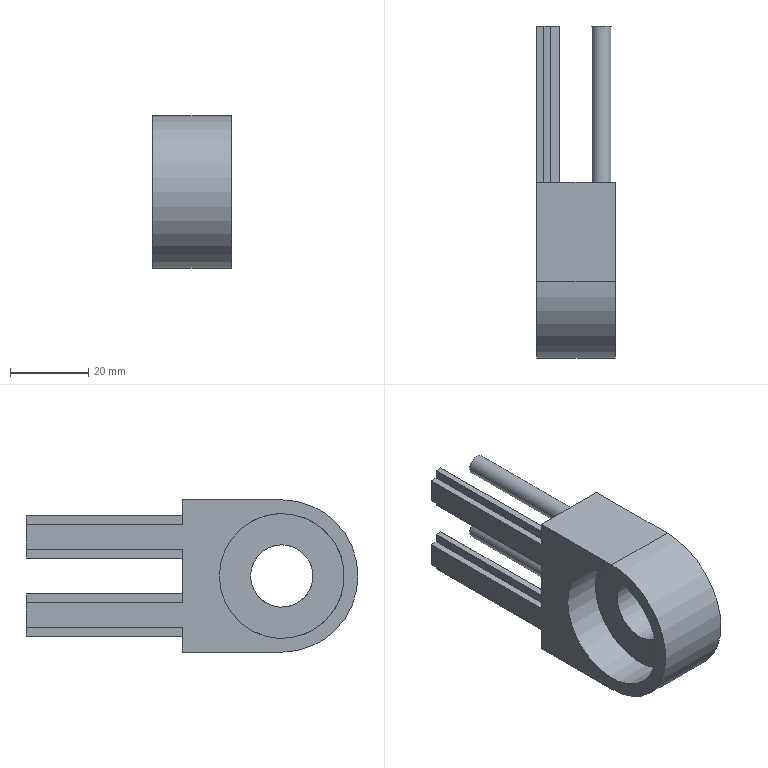Part | STEP file | YBQDJ-SSJ-4 | 1 solid | 43 faces | box 20 x 85 x 39 mm | volume 27065 mm3 | plane 32 | cylinder 11 | commonest cylinder face diameters 3 x4 4.2 x2 5 x2 16 x1 32 x1 39 x1